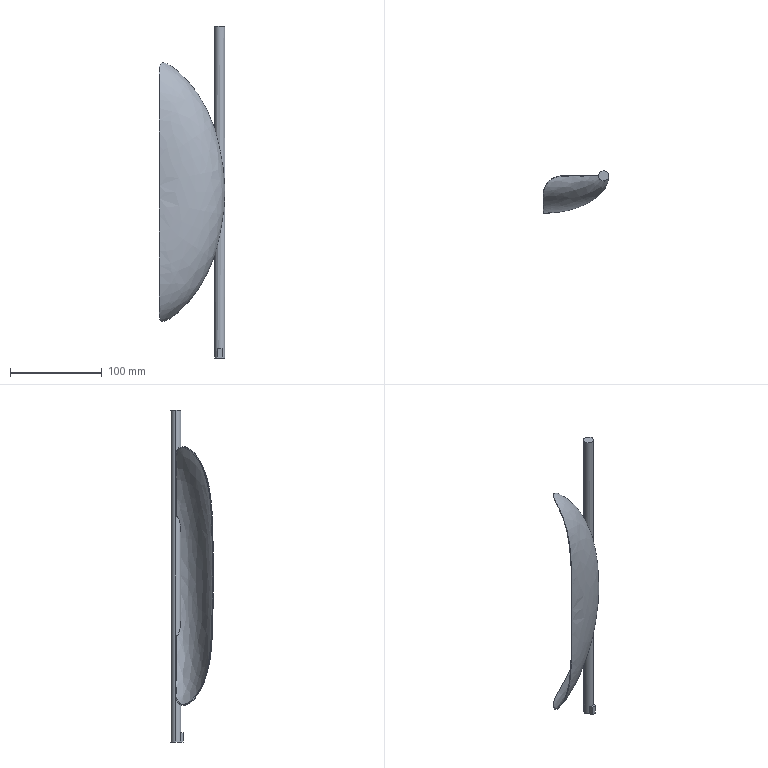Part | SolidWorks | features Attribute 3, MirrorStock 1 | 1 solid | 31 faces | box 71.359 x 45.899 x 361 mm | volume 54117 mm3 | plane 15 | spline 10 | cylinder 6 | commonest cylinder face diameters 11 x4 40 x2